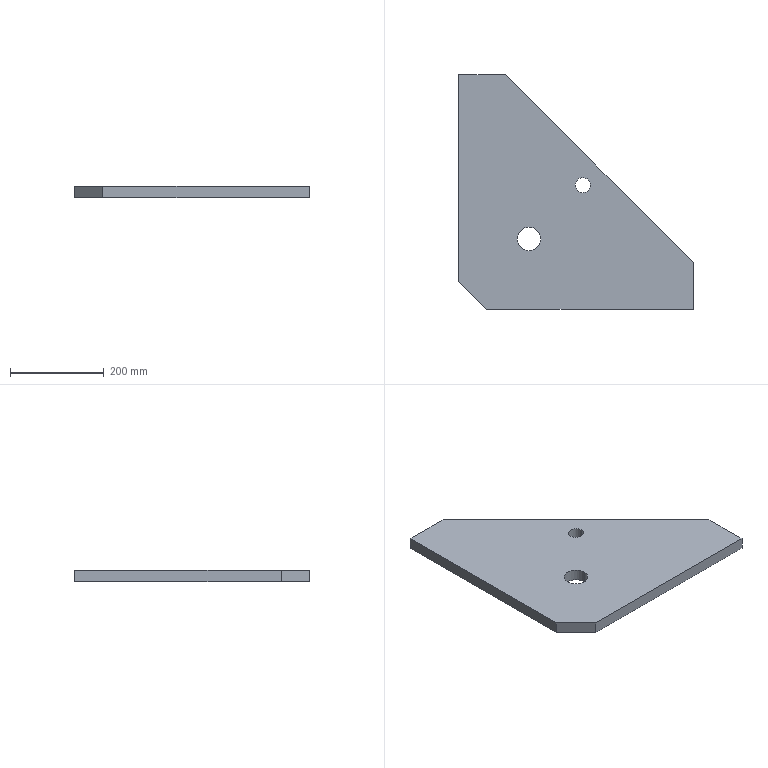Part | SolidWorks | features Chamfer 1, Cut 1, Extrusion 1, ICE 1 | 1 solid | 12 faces | box 500 x 500 x 25 mm | volume 4135806 mm3 | plane 8 | cylinder 4 | commonest cylinder face diameters 32 x2 50 x2
STEP:
#1=CARTESIAN_POINT('',(248.645,264.645,0.));
#2=VERTEX_POINT('',#1);
#3=CARTESIAN_POINT('',(280.645,264.645,0.));
#4=VERTEX_POINT('',#3);
#5=CARTESIAN_POINT('',(264.645,264.645,0.));
#6=DIRECTION('',(0.,0.,1.));
#7=DIRECTION('',(1.,0.,0.));
#8=AXIS2_PLACEMENT_3D('',#5,#6,#7);
#9=CIRCLE('',#8,16.);
#10=EDGE_CURVE('',#2,#4,#9,.T.);
#11=ORIENTED_EDGE('',*,*,#10,.F.);
#12=CARTESIAN_POINT('',(248.645,264.645,25.));
#13=VERTEX_POINT('',#12);
#14=CARTESIAN_POINT('',(248.645,264.645,0.));
#15=DIRECTION('',(0.,0.,1.));
#16=VECTOR('',#15,1000.);
#17=LINE('',#14,#16);
#18=EDGE_CURVE('',#2,#13,#17,.T.);
#19=ORIENTED_EDGE('',*,*,#18,.T.);
#20=CARTESIAN_POINT('',(280.645,264.645,25.));
#21=VERTEX_POINT('',#20);
#22=CARTESIAN_POINT('',(264.645,264.645,25.));
#23=DIRECTION('',(0.,0.,1.));
#24=DIRECTION('',(1.,0.,0.));
#25=AXIS2_PLACEMENT_3D('',#22,#23,#24);
#26=CIRCLE('',#25,16.);
#27=EDGE_CURVE('',#13,#21,#26,.T.);
#28=ORIENTED_EDGE('',*,*,#27,.T.);
#29=CARTESIAN_POINT('',(280.645,264.645,0.));
#30=DIRECTION('',(0.,0.,1.));
#31=VECTOR('',#30,1000.);
#32=LINE('',#29,#31);
#33=EDGE_CURVE('',#4,#21,#32,.T.);
#34=ORIENTED_EDGE('',*,*,#33,.F.);
#35=EDGE_LOOP('',(#11,#19,#28,#34));
#36=FACE_OUTER_BOUND('',#35,.T.);
#37=CARTESIAN_POINT('',(264.645,264.645,0.));
#38=DIRECTION('',(0.,0.,1.));
#39=DIRECTION('',(1.,0.,0.));
#40=AXIS2_PLACEMENT_3D('',#37,#38,#39);
#41=CYLINDRICAL_SURFACE('',#40,16.);
#42=ADVANCED_FACE('',(#36),#41,.F.);
#43=CARTESIAN_POINT('',(125.,150.,0.));
#44=VERTEX_POINT('',#43);
#45=CARTESIAN_POINT('',(175.,150.,0.));
#46=VERTEX_POINT('',#45);
#47=CARTESIAN_POINT('',(150.,150.,0.));
#48=DIRECTION('',(0.,0.,1.));
#49=DIRECTION('',(1.,0.,0.));
#50=AXIS2_PLACEMENT_3D('',#47,#48,#49);
#51=CIRCLE('',#50,25.);
#52=EDGE_CURVE('',#44,#46,#51,.T.);
#53=ORIENTED_EDGE('',*,*,#52,.F.);
#54=CARTESIAN_POINT('',(125.,150.,25.));
#55=VERTEX_POINT('',#54);
#56=CARTESIAN_POINT('',(125.,150.,0.));
#57=DIRECTION('',(0.,0.,1.));
#58=VECTOR('',#57,1000.);
#59=LINE('',#56,#58);
#60=EDGE_CURVE('',#44,#55,#59,.T.);
#61=ORIENTED_EDGE('',*,*,#60,.T.);
#62=CARTESIAN_POINT('',(175.,150.,25.));
#63=VERTEX_POINT('',#62);
#64=CARTESIAN_POINT('',(150.,150.,25.));
#65=DIRECTION('',(0.,0.,1.));
#66=DIRECTION('',(1.,0.,0.));
#67=AXIS2_PLACEMENT_3D('',#64,#65,#66);
#68=CIRCLE('',#67,25.);
#69=EDGE_CURVE('',#55,#63,#68,.T.);
#70=ORIENTED_EDGE('',*,*,#69,.T.);
#71=CARTESIAN_POINT('',(175.,150.,0.));
#72=DIRECTION('',(0.,0.,1.));
#73=VECTOR('',#72,1000.);
#74=LINE('',#71,#73);
#75=EDGE_CURVE('',#46,#63,#74,.T.);
#76=ORIENTED_EDGE('',*,*,#75,.F.);
#77=EDGE_LOOP('',(#53,#61,#70,#76));
#78=FACE_OUTER_BOUND('',#77,.T.);
#79=CARTESIAN_POINT('',(150.,150.,0.));
#80=DIRECTION('',(0.,0.,1.));
#81=DIRECTION('',(1.,0.,0.));
#82=AXIS2_PLACEMENT_3D('',#79,#80,#81);
#83=CYLINDRICAL_SURFACE('',#82,25.);
#84=ADVANCED_FACE('',(#78),#83,.F.);
#85=CARTESIAN_POINT('',(60.,0.,25.));
#86=VERTEX_POINT('',#85);
#87=CARTESIAN_POINT('',(500.,0.,25.));
#88=VERTEX_POINT('',#87);
#89=CARTESIAN_POINT('',(0.,0.,25.));
#90=DIRECTION('',(1.,0.,0.));
#91=VECTOR('',#90,1000.);
#92=LINE('',#89,#91);
#93=EDGE_CURVE('',#86,#88,#92,.T.);
#94=ORIENTED_EDGE('',*,*,#93,.F.);
#95=CARTESIAN_POINT('',(60.,0.,0.));
#96=VERTEX_POINT('',#95);
#97=CARTESIAN_POINT('',(60.,0.,25.));
#98=DIRECTION('',(0.,0.,-1.));
#99=VECTOR('',#98,1000.);
#100=LINE('',#97,#99);
#101=EDGE_CURVE('',#86,#96,#100,.T.);
#102=ORIENTED_EDGE('',*,*,#101,.T.);
#103=CARTESIAN_POINT('',(500.,0.,0.));
#104=VERTEX_POINT('',#103);
#105=CARTESIAN_POINT('',(0.,0.,0.));
#106=DIRECTION('',(1.,0.,0.));
#107=VECTOR('',#106,1000.);
#108=LINE('',#105,#107);
#109=EDGE_CURVE('',#96,#104,#108,.T.);
#110=ORIENTED_EDGE('',*,*,#109,.T.);
#111=CARTESIAN_POINT('',(500.,0.,25.));
#112=DIRECTION('',(0.,0.,-1.));
#113=VECTOR('',#112,1000.);
#114=LINE('',#111,#113);
#115=EDGE_CURVE('',#88,#104,#114,.T.);
#116=ORIENTED_EDGE('',*,*,#115,.F.);
#117=EDGE_LOOP('',(#94,#102,#110,#116));
#118=FACE_OUTER_BOUND('',#117,.T.);
#119=CARTESIAN_POINT('',(0.,0.,25.));
#120=DIRECTION('',(0.,1.,0.));
#121=DIRECTION('',(0.,0.,1.));
#122=AXIS2_PLACEMENT_3D('',#119,#120,#121);
#123=PLANE('',#122);
#124=ADVANCED_FACE('',(#118),#123,.F.);
#125=CARTESIAN_POINT('',(500.,100.,0.));
#126=VERTEX_POINT('',#125);
#127=CARTESIAN_POINT('',(500.,0.,0.));
#128=DIRECTION('',(0.,1.,0.));
#129=VECTOR('',#128,1000.);
#130=LINE('',#127,#129);
#131=EDGE_CURVE('',#104,#126,#130,.T.);
#132=ORIENTED_EDGE('',*,*,#131,.T.);
#133=CARTESIAN_POINT('',(500.,100.,25.));
#134=VERTEX_POINT('',#133);
#135=CARTESIAN_POINT('',(500.,100.,25.));
#136=DIRECTION('',(0.,0.,-1.));
#137=VECTOR('',#136,1000.);
#138=LINE('',#135,#137);
#139=EDGE_CURVE('',#134,#126,#138,.T.);
#140=ORIENTED_EDGE('',*,*,#139,.F.);
#141=CARTESIAN_POINT('',(500.,0.,25.));
#142=DIRECTION('',(0.,1.,0.));
#143=VECTOR('',#142,1000.);
#144=LINE('',#141,#143);
#145=EDGE_CURVE('',#88,#134,#144,.T.);
#146=ORIENTED_EDGE('',*,*,#145,.F.);
#147=ORIENTED_EDGE('',*,*,#115,.T.);
#148=EDGE_LOOP('',(#132,#140,#146,#147));
#149=FACE_OUTER_BOUND('',#148,.T.);
#150=CARTESIAN_POINT('',(500.,0.,25.));
#151=DIRECTION('',(-1.,0.,0.));
#152=DIRECTION('',(0.,0.,1.));
#153=AXIS2_PLACEMENT_3D('',#150,#151,#152);
#154=PLANE('',#153);
#155=ADVANCED_FACE('',(#149),#154,.F.);
#156=CARTESIAN_POINT('',(100.,500.,0.));
#157=VERTEX_POINT('',#156);
#158=CARTESIAN_POINT('',(100.,500.,0.));
#159=DIRECTION('',(-0.7071,0.7071,0.));
#160=VECTOR('',#159,1000.);
#161=LINE('',#158,#160);
#162=EDGE_CURVE('',#126,#157,#161,.T.);
#163=ORIENTED_EDGE('',*,*,#162,.T.);
#164=CARTESIAN_POINT('',(100.,500.,25.));
#165=VERTEX_POINT('',#164);
#166=CARTESIAN_POINT('',(100.,500.,25.));
#167=DIRECTION('',(0.,0.,-1.));
#168=VECTOR('',#167,1000.);
#169=LINE('',#166,#168);
#170=EDGE_CURVE('',#165,#157,#169,.T.);
#171=ORIENTED_EDGE('',*,*,#170,.F.);
#172=CARTESIAN_POINT('',(100.,500.,25.));
#173=DIRECTION('',(-0.7071,0.7071,0.));
#174=VECTOR('',#173,1000.);
#175=LINE('',#172,#174);
#176=EDGE_CURVE('',#134,#165,#175,.T.);
#177=ORIENTED_EDGE('',*,*,#176,.F.);
#178=ORIENTED_EDGE('',*,*,#139,.T.);
#179=EDGE_LOOP('',(#163,#171,#177,#178));
#180=FACE_OUTER_BOUND('',#179,.T.);
#181=CARTESIAN_POINT('',(100.,500.,25.));
#182=DIRECTION('',(-0.7071,-0.7071,0.));
#183=DIRECTION('',(0.7071,-0.7071,0.));
#184=AXIS2_PLACEMENT_3D('',#181,#182,#183);
#185=PLANE('',#184);
#186=ADVANCED_FACE('',(#180),#185,.F.);
#187=CARTESIAN_POINT('',(0.,500.,0.));
#188=VERTEX_POINT('',#187);
#189=CARTESIAN_POINT('',(0.,500.,0.));
#190=DIRECTION('',(-1.,0.,0.));
#191=VECTOR('',#190,1000.);
#192=LINE('',#189,#191);
#193=EDGE_CURVE('',#157,#188,#192,.T.);
#194=ORIENTED_EDGE('',*,*,#193,.T.);
#195=CARTESIAN_POINT('',(0.,500.,25.));
#196=VERTEX_POINT('',#195);
#197=CARTESIAN_POINT('',(0.,500.,25.));
#198=DIRECTION('',(0.,0.,-1.));
#199=VECTOR('',#198,1000.);
#200=LINE('',#197,#199);
#201=EDGE_CURVE('',#196,#188,#200,.T.);
#202=ORIENTED_EDGE('',*,*,#201,.F.);
#203=CARTESIAN_POINT('',(0.,500.,25.));
#204=DIRECTION('',(-1.,0.,0.));
#205=VECTOR('',#204,1000.);
#206=LINE('',#203,#205);
#207=EDGE_CURVE('',#165,#196,#206,.T.);
#208=ORIENTED_EDGE('',*,*,#207,.F.);
#209=ORIENTED_EDGE('',*,*,#170,.T.);
#210=EDGE_LOOP('',(#194,#202,#208,#209));
#211=FACE_OUTER_BOUND('',#210,.T.);
#212=CARTESIAN_POINT('',(0.,500.,25.));
#213=DIRECTION('',(0.,-1.,0.));
#214=DIRECTION('',(0.,0.,-1.));
#215=AXIS2_PLACEMENT_3D('',#212,#213,#214);
#216=PLANE('',#215);
#217=ADVANCED_FACE('',(#211),#216,.F.);
#218=CARTESIAN_POINT('',(0.,60.,0.));
#219=VERTEX_POINT('',#218);
#220=CARTESIAN_POINT('',(0.,0.,0.));
#221=DIRECTION('',(0.,-1.,0.));
#222=VECTOR('',#221,1000.);
#223=LINE('',#220,#222);
#224=EDGE_CURVE('',#188,#219,#223,.T.);
#225=ORIENTED_EDGE('',*,*,#224,.T.);
#226=CARTESIAN_POINT('',(0.,60.,25.));
#227=VERTEX_POINT('',#226);
#228=CARTESIAN_POINT('',(0.,60.,25.));
#229=DIRECTION('',(0.,0.,1.));
#230=VECTOR('',#229,1000.);
#231=LINE('',#228,#230);
#232=EDGE_CURVE('',#219,#227,#231,.T.);
#233=ORIENTED_EDGE('',*,*,#232,.T.);
#234=CARTESIAN_POINT('',(0.,0.,25.));
#235=DIRECTION('',(0.,-1.,0.));
#236=VECTOR('',#235,1000.);
#237=LINE('',#234,#236);
#238=EDGE_CURVE('',#196,#227,#237,.T.);
#239=ORIENTED_EDGE('',*,*,#238,.F.);
#240=ORIENTED_EDGE('',*,*,#201,.T.);
#241=EDGE_LOOP('',(#225,#233,#239,#240));
#242=FACE_OUTER_BOUND('',#241,.T.);
#243=CARTESIAN_POINT('',(0.,0.,25.));
#244=DIRECTION('',(1.,0.,0.));
#245=DIRECTION('',(0.,0.,-1.));
#246=AXIS2_PLACEMENT_3D('',#243,#244,#245);
#247=PLANE('',#246);
#248=ADVANCED_FACE('',(#242),#247,.F.);
#249=CARTESIAN_POINT('',(264.645,264.645,25.));
#250=DIRECTION('',(0.,0.,1.));
#251=DIRECTION('',(1.,0.,0.));
#252=AXIS2_PLACEMENT_3D('',#249,#250,#251);
#253=CIRCLE('',#252,16.);
#254=EDGE_CURVE('',#21,#13,#253,.T.);
#255=ORIENTED_EDGE('',*,*,#254,.F.);
#256=ORIENTED_EDGE('',*,*,#27,.F.);
#257=EDGE_LOOP('',(#255,#256));
#258=FACE_BOUND('',#257,.T.);
#259=CARTESIAN_POINT('',(150.,150.,25.));
#260=DIRECTION('',(0.,0.,1.));
#261=DIRECTION('',(1.,0.,0.));
#262=AXIS2_PLACEMENT_3D('',#259,#260,#261);
#263=CIRCLE('',#262,25.);
#264=EDGE_CURVE('',#63,#55,#263,.T.);
#265=ORIENTED_EDGE('',*,*,#264,.F.);
#266=ORIENTED_EDGE('',*,*,#69,.F.);
#267=EDGE_LOOP('',(#265,#266));
#268=FACE_BOUND('',#267,.T.);
#269=ORIENTED_EDGE('',*,*,#238,.T.);
#270=CARTESIAN_POINT('',(30.,30.,25.));
#271=DIRECTION('',(0.7071,-0.7071,0.));
#272=VECTOR('',#271,1000.);
#273=LINE('',#270,#272);
#274=EDGE_CURVE('',#227,#86,#273,.T.);
#275=ORIENTED_EDGE('',*,*,#274,.T.);
#276=ORIENTED_EDGE('',*,*,#93,.T.);
#277=ORIENTED_EDGE('',*,*,#145,.T.);
#278=ORIENTED_EDGE('',*,*,#176,.T.);
#279=ORIENTED_EDGE('',*,*,#207,.T.);
#280=EDGE_LOOP('',(#269,#275,#276,#277,#278,#279));
#281=FACE_OUTER_BOUND('',#280,.T.);
#282=CARTESIAN_POINT('',(0.,0.,25.));
#283=DIRECTION('',(0.,0.,1.));
#284=DIRECTION('',(1.,0.,0.));
#285=AXIS2_PLACEMENT_3D('',#282,#283,#284);
#286=PLANE('',#285);
#287=ADVANCED_FACE('',(#258,#268,#281),#286,.T.);
#288=CARTESIAN_POINT('',(264.645,264.645,0.));
#289=DIRECTION('',(0.,0.,1.));
#290=DIRECTION('',(1.,0.,0.));
#291=AXIS2_PLACEMENT_3D('',#288,#289,#290);
#292=CIRCLE('',#291,16.);
#293=EDGE_CURVE('',#4,#2,#292,.T.);
#294=ORIENTED_EDGE('',*,*,#293,.T.);
#295=ORIENTED_EDGE('',*,*,#10,.T.);
#296=EDGE_LOOP('',(#294,#295));
#297=FACE_BOUND('',#296,.T.);
#298=CARTESIAN_POINT('',(150.,150.,0.));
#299=DIRECTION('',(0.,0.,1.));
#300=DIRECTION('',(1.,0.,0.));
#301=AXIS2_PLACEMENT_3D('',#298,#299,#300);
#302=CIRCLE('',#301,25.);
#303=EDGE_CURVE('',#46,#44,#302,.T.);
#304=ORIENTED_EDGE('',*,*,#303,.T.);
#305=ORIENTED_EDGE('',*,*,#52,.T.);
#306=EDGE_LOOP('',(#304,#305));
#307=FACE_BOUND('',#306,.T.);
#308=ORIENTED_EDGE('',*,*,#109,.F.);
#309=CARTESIAN_POINT('',(60.,0.,0.));
#310=DIRECTION('',(-0.7071,0.7071,0.));
#311=VECTOR('',#310,1000.);
#312=LINE('',#309,#311);
#313=EDGE_CURVE('',#96,#219,#312,.T.);
#314=ORIENTED_EDGE('',*,*,#313,.T.);
#315=ORIENTED_EDGE('',*,*,#224,.F.);
#316=ORIENTED_EDGE('',*,*,#193,.F.);
#317=ORIENTED_EDGE('',*,*,#162,.F.);
#318=ORIENTED_EDGE('',*,*,#131,.F.);
#319=EDGE_LOOP('',(#308,#314,#315,#316,#317,#318));
#320=FACE_OUTER_BOUND('',#319,.T.);
#321=CARTESIAN_POINT('',(0.,0.,0.));
#322=DIRECTION('',(0.,0.,1.));
#323=DIRECTION('',(1.,0.,0.));
#324=AXIS2_PLACEMENT_3D('',#321,#322,#323);
#325=PLANE('',#324);
#326=ADVANCED_FACE('',(#297,#307,#320),#325,.F.);
#327=ORIENTED_EDGE('',*,*,#60,.F.);
#328=ORIENTED_EDGE('',*,*,#303,.F.);
#329=ORIENTED_EDGE('',*,*,#75,.T.);
#330=ORIENTED_EDGE('',*,*,#264,.T.);
#331=EDGE_LOOP('',(#327,#328,#329,#330));
#332=FACE_OUTER_BOUND('',#331,.T.);
#333=CARTESIAN_POINT('',(150.,150.,0.));
#334=DIRECTION('',(0.,0.,1.));
#335=DIRECTION('',(1.,0.,0.));
#336=AXIS2_PLACEMENT_3D('',#333,#334,#335);
#337=CYLINDRICAL_SURFACE('',#336,25.);
#338=ADVANCED_FACE('',(#332),#337,.F.);
#339=ORIENTED_EDGE('',*,*,#274,.F.);
#340=ORIENTED_EDGE('',*,*,#232,.F.);
#341=ORIENTED_EDGE('',*,*,#313,.F.);
#342=ORIENTED_EDGE('',*,*,#101,.F.);
#343=EDGE_LOOP('',(#339,#340,#341,#342));
#344=FACE_OUTER_BOUND('',#343,.T.);
#345=CARTESIAN_POINT('',(60.,0.,25.));
#346=DIRECTION('',(0.7071,0.7071,0.));
#347=DIRECTION('',(0.,0.,-1.));
#348=AXIS2_PLACEMENT_3D('',#345,#346,#347);
#349=PLANE('',#348);
#350=ADVANCED_FACE('',(#344),#349,.F.);
#351=ORIENTED_EDGE('',*,*,#18,.F.);
#352=ORIENTED_EDGE('',*,*,#293,.F.);
#353=ORIENTED_EDGE('',*,*,#33,.T.);
#354=ORIENTED_EDGE('',*,*,#254,.T.);
#355=EDGE_LOOP('',(#351,#352,#353,#354));
#356=FACE_OUTER_BOUND('',#355,.T.);
#357=CARTESIAN_POINT('',(264.645,264.645,0.));
#358=DIRECTION('',(0.,0.,1.));
#359=DIRECTION('',(1.,0.,0.));
#360=AXIS2_PLACEMENT_3D('',#357,#358,#359);
#361=CYLINDRICAL_SURFACE('',#360,16.);
#362=ADVANCED_FACE('',(#356),#361,.F.);
#363=CLOSED_SHELL('',(#42,#84,#124,#155,#186,#217,#248,#287,#326,#338,#350,#362));
#364=MANIFOLD_SOLID_BREP('',#363);
#365=CARTESIAN_POINT('',(0.,0.,0.));
#366=DIRECTION('',(0.,0.,1.));
#367=DIRECTION('',(1.,0.,0.));
#368=AXIS2_PLACEMENT_3D('',#365,#366,#367);
#369=(LENGTH_UNIT()NAMED_UNIT(*)SI_UNIT(.MILLI.,.METRE.));
#370=UNCERTAINTY_MEASURE_WITH_UNIT(LENGTH_MEASURE(0.00001),#369,'','');
#371=(NAMED_UNIT(*)PLANE_ANGLE_UNIT()SI_UNIT($,.RADIAN.));
#372=(NAMED_UNIT(*)SI_UNIT($,.STERADIAN.)SOLID_ANGLE_UNIT());
#373=(GEOMETRIC_REPRESENTATION_CONTEXT(3)GLOBAL_UNCERTAINTY_ASSIGNED_CONTEXT((#370))GLOBAL_UNIT_ASSIGNED_CONTEXT((#369,#371,#372))REPRESENTATION_CONTEXT('',''));
#374=ADVANCED_BREP_SHAPE_REPRESENTATION('',(#364,#368),#373);